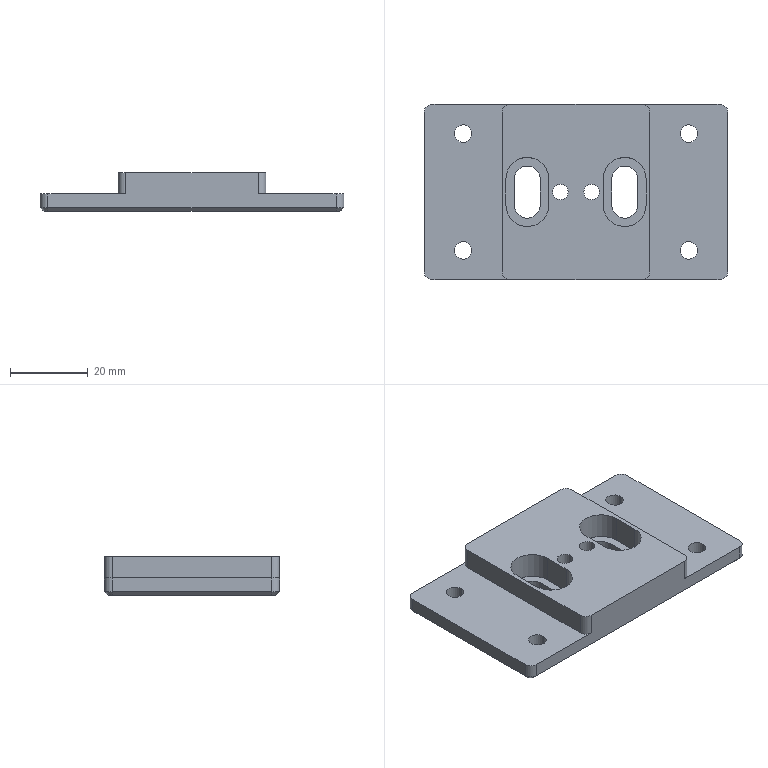NC program | NX | posted with a generic post | part box 78 x 45 x 10 mm
Lines 3249 to 4289 of 4289:
(ZLEVEL_PROFILE_COPY_COPY_1_COPY_1_COPY , TOOL : D4)
N6466 T04 M6
N6468 G54
N6470 G17 G0 G90 X-11.945 Y-4.566 S9500 M3
N6472 G43 Z30. H4
N6474 Z-5.3
N6476 G94 G1 X-11.757 Y-4.479 Z-5.311 F1400.
N6478 X-11.443 Y-4.173 Z-5.334
N6480 X-11.285 Y-3.891 Z-5.351
N6482 X-11.2 Y-3.562 Z-5.369
N6484 Y3.562 Z-5.742
N6486 X-11.285 Y3.891 Z-5.76
N6488 X-11.369 Y4.042 Z-5.769
N6490 X-11.449 Y4.182 Z-5.777
N6492 X-11.764 Y4.484 Z-5.8
N6494 X-12.16 Y4.665 Z-5.823
N6496 X-12.594 Y4.707 Z-5.846
N6498 X-13.017 Y4.604 Z-5.869
N6500 X-13.16 Y4.52 Z-5.877
N6502 X-13.299 Y4.438 Z-5.886
N6504 X-13.553 Y4.179 Z-5.905
N6506 X-13.636 Y4.032 Z-5.914
N6508 X-13.715 Y3.891 Z-5.922
N6510 X-13.8 Y3.562 Z-5.94
N6512 Y-3.562 Z-6.313
N6514 X-13.715 Y-3.891 Z-6.331
N6516 X-13.631 Y-4.041 Z-6.34
N6518 X-13.551 Y-4.182 Z-6.349
N6520 X-13.298 Y-4.439 Z-6.367
N6522 X-13.156 Y-4.522 Z-6.376
N6524 X-13.017 Y-4.604 Z-6.384
N6526 X-12.591 Y-4.707 Z-6.407
N6528 X-12.155 Y-4.664 Z-6.43
N6530 X-11.757 Y-4.479 Z-6.453
N6532 X-11.443 Y-4.173 Z-6.476
N6534 X-11.285 Y-3.891 Z-6.493
N6536 X-11.2 Y-3.562 Z-6.511
N6538 Y3.562 Z-6.884
N6540 X-11.285 Y3.891 Z-6.902
N6542 X-11.369 Y4.042 Z-6.911
N6544 X-11.449 Y4.182 Z-6.92
N6546 X-11.764 Y4.484 Z-6.943
N6548 X-12.16 Y4.665 Z-6.965
N6550 X-12.594 Y4.707 Z-6.988
N6552 X-13.017 Y4.604 Z-7.011
N6554 X-13.16 Y4.52 Z-7.02
N6556 X-13.299 Y4.438 Z-7.028
N6558 X-13.553 Y4.179 Z-7.047
N6560 X-13.636 Y4.032 Z-7.056
N6562 X-13.715 Y3.891 Z-7.065
N6564 X-13.8 Y3.562 Z-7.082
N6566 Y3.4 Z-7.091
N6568 Y-3.4
N6570 G3 X-12.5 Y-4.7 R1.3
N6572 X-11.2 Y-3.4 R1.3
N6574 G1 Y3.4
N6576 G3 X-12.5 Y4.7 R1.3
N6578 X-13.8 Y3.4 R1.3
N6580 G1 Y-3.215 Z-7.209
N6582 X-13.799 Y-3.356 Z-7.211
N6584 X-13.788 Y-3.495 Z-7.214
N6586 X-13.772 Y-3.635 Z-7.216
N6588 X-13.737 Y-3.785 Z-7.219
N6590 X-13.692 Y-3.902 Z-7.221
N6592 X-13.612 Y-4.058 Z-7.224
N6594 X-13.557 Y-4.147 Z-7.226
N6596 X-13.465 Y-4.262 Z-7.229
N6598 X-13.37 Y-4.355 Z-7.231
N6600 X-13.229 Y-4.467 Z-7.235
N6602 X-13.146 Y-4.523 Z-7.236
N6604 X-13.018 Y-4.585 Z-7.239
N6606 X-12.889 Y-4.632 Z-7.241
N6608 X-12.721 Y-4.673 Z-7.244
N6610 X-12.615 Y-4.689 Z-7.246
N6612 X-12.464 Y-4.692 Z-7.249
N6614 X-12.336 Y-4.682 Z-7.251
N6616 X-12.171 Y-4.651 Z-7.254
N6618 X-12.064 Y-4.617 Z-7.256
N6620 X-11.911 Y-4.55 Z-7.259
N6622 X-11.813 Y-4.495 Z-7.261
N6624 X-11.682 Y-4.404 Z-7.264
N6626 X-11.593 Y-4.322 Z-7.266
N6628 X-11.477 Y-4.189 Z-7.27
N6630 X-11.416 Y-4.106 Z-7.271
N6632 X-11.345 Y-3.984 Z-7.274
N6634 X-11.291 Y-3.856 Z-7.276
N6636 X-11.238 Y-3.679 Z-7.28
N6638 X-11.214 Y-3.587 Z-7.282
N6640 X-11.201 Y-3.447 Z-7.284
N6642 X-11.2 Y-3.306 Z-7.287
N6644 Y2.042 Z-7.382
N6646 Y3.4
N6648 G3 X-12.5 Y4.7 R1.3
N6650 X-13.8 Y3.4 R1.3
N6652 G1 Y-3.215 Z-7.5
N6654 X-13.799 Y-3.356 Z-7.502
N6656 X-13.788 Y-3.495 Z-7.505
N6658 X-13.772 Y-3.635 Z-7.507
N6660 X-13.737 Y-3.785 Z-7.51
N6662 X-13.692 Y-3.902 Z-7.512
N6664 X-13.612 Y-4.058 Z-7.515
N6666 X-13.557 Y-4.147 Z-7.517
N6668 X-13.465 Y-4.262 Z-7.52
N6670 X-13.37 Y-4.355 Z-7.522
N6672 X-13.229 Y-4.467 Z-7.525
N6674 X-13.146 Y-4.523 Z-7.527
N6676 X-13.018 Y-4.585 Z-7.53
N6678 X-12.889 Y-4.632 Z-7.532
N6680 X-12.721 Y-4.673 Z-7.535
N6682 X-12.615 Y-4.689 Z-7.537
N6684 X-12.464 Y-4.692 Z-7.54
N6686 X-12.336 Y-4.682 Z-7.542
N6688 X-12.171 Y-4.651 Z-7.545
N6690 X-12.064 Y-4.617 Z-7.547
N6692 X-11.911 Y-4.55 Z-7.55
N6694 X-11.813 Y-4.495 Z-7.552
N6696 X-11.682 Y-4.404 Z-7.555
N6698 X-11.593 Y-4.322 Z-7.557
N6700 X-11.477 Y-4.189 Z-7.561
N6702 X-11.416 Y-4.106 Z-7.562
N6704 X-11.345 Y-3.984 Z-7.565
N6706 X-11.291 Y-3.856 Z-7.567
N6708 X-11.238 Y-3.679 Z-7.571
N6710 X-11.214 Y-3.587 Z-7.572
N6712 X-11.201 Y-3.447 Z-7.575
N6714 X-11.2 Y-3.306 Z-7.577
N6716 Y2.042 Z-7.673
N6718 Y3.4
N6720 G3 X-12.5 Y4.7 R1.3
N6722 X-13.8 Y3.4 R1.3
N6724 G1 Y-3.215 Z-7.791
N6726 X-13.799 Y-3.356 Z-7.793
N6728 X-13.788 Y-3.495 Z-7.796
N6730 X-13.772 Y-3.635 Z-7.798
N6732 X-13.736 Y-3.785 Z-7.801
N6734 X-13.692 Y-3.902 Z-7.803
N6736 X-13.612 Y-4.058 Z-7.806
N6738 X-13.557 Y-4.147 Z-7.808
N6740 X-13.465 Y-4.262 Z-7.811
N6742 X-13.37 Y-4.355 Z-7.813
N6744 X-13.229 Y-4.467 Z-7.816
N6746 X-13.146 Y-4.523 Z-7.818
N6748 X-13.018 Y-4.585 Z-7.821
N6750 X-12.889 Y-4.632 Z-7.823
N6752 X-12.721 Y-4.673 Z-7.826
N6754 X-12.615 Y-4.689 Z-7.828
N6756 X-12.464 Y-4.692 Z-7.831
N6758 X-12.336 Y-4.682 Z-7.833
N6760 X-12.171 Y-4.651 Z-7.836
N6762 X-12.064 Y-4.617 Z-7.838
N6764 X-11.911 Y-4.55 Z-7.841
N6766 X-11.813 Y-4.495 Z-7.843
N6768 X-11.682 Y-4.404 Z-7.846
N6770 X-11.593 Y-4.322 Z-7.848
N6772 X-11.477 Y-4.189 Z-7.851
N6774 X-11.416 Y-4.106 Z-7.853
N6776 X-11.346 Y-3.984 Z-7.856
N6778 X-11.291 Y-3.856 Z-7.858
N6780 X-11.238 Y-3.679 Z-7.862
N6782 X-11.214 Y-3.587 Z-7.863
N6784 X-11.201 Y-3.447 Z-7.866
N6786 X-11.2 Y-3.306 Z-7.868
N6788 Y2.042 Z-7.964
N6790 Y3.4
N6792 G3 X-12.5 Y4.7 R1.3
N6794 X-13.8 Y3.4 R1.3
N6796 G1 Y-3.215 Z-8.082
N6798 X-13.799 Y-3.356 Z-8.084
N6800 X-13.788 Y-3.495 Z-8.087
N6802 X-13.772 Y-3.635 Z-8.089
N6804 X-13.736 Y-3.785 Z-8.092
N6806 X-13.692 Y-3.902 Z-8.094
N6808 X-13.612 Y-4.058 Z-8.097
N6810 X-13.557 Y-4.147 Z-8.099
N6812 X-13.465 Y-4.262 Z-8.102
N6814 X-13.37 Y-4.355 Z-8.104
N6816 X-13.229 Y-4.467 Z-8.107
N6818 X-13.146 Y-4.523 Z-8.109
N6820 X-13.018 Y-4.585 Z-8.112
N6822 X-12.889 Y-4.632 Z-8.114
N6824 X-12.721 Y-4.673 Z-8.117
N6826 X-12.615 Y-4.689 Z-8.119
N6828 X-12.464 Y-4.692 Z-8.122
N6830 X-12.336 Y-4.682 Z-8.124
N6832 X-12.171 Y-4.651 Z-8.127
N6834 X-12.064 Y-4.617 Z-8.129
N6836 X-11.911 Y-4.55 Z-8.132
N6838 X-11.813 Y-4.495 Z-8.134
N6840 X-11.682 Y-4.404 Z-8.137
N6842 X-11.593 Y-4.322 Z-8.139
N6844 X-11.477 Y-4.189 Z-8.142
N6846 X-11.416 Y-4.106 Z-8.144
N6848 X-11.346 Y-3.984 Z-8.147
N6850 X-11.291 Y-3.856 Z-8.149
N6852 X-11.238 Y-3.679 Z-8.153
N6854 X-11.214 Y-3.587 Z-8.154
N6856 X-11.201 Y-3.447 Z-8.157
N6858 X-11.2 Y-3.306 Z-8.159
N6860 Y2.042 Z-8.255
N6862 Y3.4
N6864 G3 X-12.5 Y4.7 R1.3
N6866 X-13.8 Y3.4 R1.3
N6868 G1 Y-3.215 Z-8.372
N6870 X-13.799 Y-3.356 Z-8.375
N6872 X-13.788 Y-3.495 Z-8.377
N6874 X-13.772 Y-3.635 Z-8.38
N6876 X-13.736 Y-3.785 Z-8.383
N6878 X-13.692 Y-3.902 Z-8.385
N6880 X-13.612 Y-4.058 Z-8.388
N6882 X-13.557 Y-4.147 Z-8.39
N6884 X-13.465 Y-4.262 Z-8.393
N6886 X-13.37 Y-4.355 Z-8.395
N6888 X-13.229 Y-4.467 Z-8.398
N6890 X-13.146 Y-4.523 Z-8.4
N6892 X-13.018 Y-4.585 Z-8.403
N6894 X-12.889 Y-4.632 Z-8.405
N6896 X-12.721 Y-4.673 Z-8.408
N6898 X-12.615 Y-4.689 Z-8.41
N6900 X-12.464 Y-4.692 Z-8.413
N6902 X-12.336 Y-4.682 Z-8.415
N6904 X-12.171 Y-4.651 Z-8.418
N6906 X-12.064 Y-4.617 Z-8.42
N6908 X-11.911 Y-4.55 Z-8.423
N6910 X-11.813 Y-4.495 Z-8.425
N6912 X-11.682 Y-4.404 Z-8.428
N6914 X-11.593 Y-4.322 Z-8.43
N6916 X-11.477 Y-4.189 Z-8.433
N6918 X-11.416 Y-4.106 Z-8.435
N6920 X-11.346 Y-3.984 Z-8.438
N6922 X-11.291 Y-3.856 Z-8.44
N6924 X-11.238 Y-3.679 Z-8.443
N6926 X-11.214 Y-3.587 Z-8.445
N6928 X-11.201 Y-3.447 Z-8.448
N6930 X-11.2 Y-3.306 Z-8.45
N6932 Y2.042 Z-8.545
N6934 Y3.4
N6936 G3 X-12.5 Y4.7 R1.3
N6938 X-13.8 Y3.4 R1.3
N6940 G1 Y-3.215 Z-8.663
N6942 X-13.799 Y-3.356 Z-8.666
N6944 X-13.788 Y-3.495 Z-8.668
N6946 X-13.772 Y-3.635 Z-8.671
N6948 X-13.736 Y-3.785 Z-8.674
N6950 X-13.692 Y-3.902 Z-8.676
N6952 X-13.612 Y-4.058 Z-8.679
N6954 X-13.557 Y-4.147 Z-8.681
N6956 X-13.465 Y-4.262 Z-8.684
N6958 X-13.37 Y-4.355 Z-8.686
N6960 X-13.229 Y-4.467 Z-8.689
N6962 X-13.146 Y-4.523 Z-8.691
N6964 X-13.018 Y-4.585 Z-8.693
N6966 X-12.889 Y-4.632 Z-8.696
N6968 X-12.721 Y-4.673 Z-8.699
N6970 X-12.615 Y-4.689 Z-8.701
N6972 X-12.464 Y-4.692 Z-8.704
N6974 X-12.336 Y-4.682 Z-8.706
N6976 X-12.171 Y-4.651 Z-8.709
N6978 X-12.064 Y-4.617 Z-8.711
N6980 X-11.911 Y-4.55 Z-8.714
N6982 X-11.813 Y-4.495 Z-8.716
N6984 X-11.682 Y-4.404 Z-8.719
N6986 X-11.593 Y-4.322 Z-8.721
N6988 X-11.477 Y-4.189 Z-8.724
N6990 X-11.416 Y-4.106 Z-8.726
N6992 X-11.346 Y-3.984 Z-8.729
N6994 X-11.291 Y-3.856 Z-8.731
N6996 X-11.238 Y-3.679 Z-8.734
N6998 X-11.214 Y-3.587 Z-8.736
N7000 X-11.201 Y-3.447 Z-8.739
N7002 X-11.2 Y-3.306 Z-8.741
N7004 Y2.042 Z-8.836
N7006 Y3.4
N7008 G3 X-12.5 Y4.7 R1.3
N7010 X-13.8 Y3.4 R1.3
N7012 G1 Y-3.215 Z-8.954
N7014 X-13.799 Y-3.356 Z-8.957
N7016 X-13.788 Y-3.495 Z-8.959
N7018 X-13.772 Y-3.635 Z-8.962
N7020 X-13.736 Y-3.785 Z-8.965
N7022 X-13.692 Y-3.902 Z-8.967
N7024 X-13.612 Y-4.058 Z-8.97
N7026 X-13.557 Y-4.147 Z-8.972
N7028 X-13.465 Y-4.262 Z-8.974
N7030 X-13.37 Y-4.355 Z-8.977
N7032 X-13.229 Y-4.467 Z-8.98
N7034 X-13.146 Y-4.523 Z-8.982
N7036 X-13.018 Y-4.585 Z-8.984
N7038 X-12.889 Y-4.632 Z-8.987
N7040 X-12.721 Y-4.673 Z-8.99
N7042 X-12.615 Y-4.689 Z-8.992
N7044 X-12.464 Y-4.692 Z-8.995
N7046 X-12.336 Y-4.682 Z-8.997
N7048 X-12.171 Y-4.651 Z-9.
N7050 X-12.064 Y-4.617 Z-9.002
N7052 X-11.911 Y-4.55 Z-9.005
N7054 X-11.813 Y-4.495 Z-9.007
N7056 X-11.682 Y-4.404 Z-9.01
N7058 X-11.593 Y-4.322 Z-9.012
N7060 X-11.477 Y-4.19 Z-9.015
N7062 X-11.416 Y-4.106 Z-9.017
N7064 X-11.346 Y-3.984 Z-9.019
N7066 X-11.291 Y-3.856 Z-9.022
N7068 X-11.238 Y-3.679 Z-9.025
N7070 X-11.214 Y-3.587 Z-9.027
N7072 X-11.201 Y-3.447 Z-9.029
N7074 X-11.2 Y-3.306 Z-9.032
N7076 Y2.042 Z-9.127
N7078 Y3.4
N7080 G3 X-12.5 Y4.7 R1.3
N7082 X-13.8 Y3.4 R1.3
N7084 G1 Y-3.215 Z-9.245
N7086 X-13.799 Y-3.356 Z-9.248
N7088 X-13.788 Y-3.495 Z-9.25
N7090 X-13.772 Y-3.635 Z-9.253
N7092 X-13.736 Y-3.785 Z-9.255
N7094 X-13.692 Y-3.902 Z-9.258
N7096 X-13.612 Y-4.058 Z-9.261
N7098 X-13.557 Y-4.147 Z-9.263
N7100 X-13.465 Y-4.262 Z-9.265
N7102 X-13.37 Y-4.355 Z-9.268
N7104 X-13.229 Y-4.467 Z-9.271
N7106 X-13.146 Y-4.523 Z-9.273
N7108 X-13.018 Y-4.585 Z-9.275
N7110 X-12.889 Y-4.632 Z-9.278
N7112 X-12.721 Y-4.673 Z-9.281
N7114 X-12.615 Y-4.689 Z-9.283
N7116 X-12.464 Y-4.692 Z-9.285
N7118 X-12.336 Y-4.682 Z-9.288
N7120 X-12.171 Y-4.651 Z-9.291
N7122 X-12.064 Y-4.617 Z-9.293
N7124 X-11.911 Y-4.55 Z-9.296
N7126 X-11.813 Y-4.495 Z-9.298
N7128 X-11.682 Y-4.404 Z-9.301
N7130 X-11.593 Y-4.322 Z-9.303
N7132 X-11.477 Y-4.19 Z-9.306
N7134 X-11.416 Y-4.106 Z-9.308
N7136 X-11.346 Y-3.984 Z-9.31
N7138 X-11.291 Y-3.856 Z-9.313
N7140 X-11.238 Y-3.679 Z-9.316
N7142 X-11.214 Y-3.587 Z-9.318
N7144 X-11.201 Y-3.447 Z-9.32
N7146 X-11.2 Y-3.306 Z-9.323
N7148 Y2.042 Z-9.418
N7150 Y3.4
N7152 G3 X-12.5 Y4.7 R1.3
N7154 X-13.8 Y3.4 R1.3
N7156 G1 Y-3.215 Z-9.536
N7158 X-13.799 Y-3.356 Z-9.539
N7160 X-13.788 Y-3.495 Z-9.541
N7162 X-13.772 Y-3.635 Z-9.544
N7164 X-13.736 Y-3.785 Z-9.546
N7166 X-13.692 Y-3.902 Z-9.549
N7168 X-13.612 Y-4.058 Z-9.552
N7170 X-13.557 Y-4.147 Z-9.554
N7172 X-13.465 Y-4.262 Z-9.556
N7174 X-13.37 Y-4.355 Z-9.559
N7176 X-13.229 Y-4.467 Z-9.562
N7178 X-13.146 Y-4.523 Z-9.564
N7180 X-13.018 Y-4.585 Z-9.566
N7182 X-12.889 Y-4.632 Z-9.569
N7184 X-12.721 Y-4.673 Z-9.572
N7186 X-12.615 Y-4.689 Z-9.574
N7188 X-12.464 Y-4.692 Z-9.576
N7190 X-12.336 Y-4.682 Z-9.579
N7192 X-12.171 Y-4.651 Z-9.582
N7194 X-12.064 Y-4.617 Z-9.584
N7196 X-11.911 Y-4.55 Z-9.587
N7198 X-11.813 Y-4.495 Z-9.589
N7200 X-11.682 Y-4.404 Z-9.592
N7202 X-11.593 Y-4.322 Z-9.594
N7204 X-11.477 Y-4.19 Z-9.597
N7206 X-11.416 Y-4.106 Z-9.599
N7208 X-11.346 Y-3.985 Z-9.601
N7210 X-11.291 Y-3.856 Z-9.604
N7212 X-11.238 Y-3.679 Z-9.607
N7214 X-11.214 Y-3.587 Z-9.609
N7216 X-11.201 Y-3.447 Z-9.611
N7218 X-11.2 Y-3.306 Z-9.614
N7220 Y2.042 Z-9.709
N7222 Y3.4
N7224 G3 X-12.5 Y4.7 R1.3
N7226 X-13.8 Y3.4 R1.3
N7228 G1 Y-3.215 Z-9.827
N7230 X-13.799 Y-3.356 Z-9.829
N7232 X-13.788 Y-3.495 Z-9.832
N7234 X-13.772 Y-3.635 Z-9.834
N7236 X-13.736 Y-3.785 Z-9.837
N7238 X-13.692 Y-3.902 Z-9.839
N7240 X-13.612 Y-4.058 Z-9.843
N7242 X-13.557 Y-4.147 Z-9.845
N7244 X-13.465 Y-4.262 Z-9.847
N7246 X-13.37 Y-4.355 Z-9.85
N7248 X-13.229 Y-4.467 Z-9.853
N7250 X-13.146 Y-4.523 Z-9.855
N7252 X-13.018 Y-4.585 Z-9.857
N7254 X-12.889 Y-4.632 Z-9.86
N7256 X-12.721 Y-4.673 Z-9.863
N7258 X-12.615 Y-4.689 Z-9.865
N7260 X-12.464 Y-4.692 Z-9.867
N7262 X-12.336 Y-4.682 Z-9.87
N7264 X-12.171 Y-4.651 Z-9.873
N7266 X-12.064 Y-4.617 Z-9.875
N7268 X-11.911 Y-4.55 Z-9.878
N7270 X-11.813 Y-4.495 Z-9.88
N7272 X-11.682 Y-4.404 Z-9.882
N7274 X-11.593 Y-4.322 Z-9.885
N7276 X-11.478 Y-4.19 Z-9.888
N7278 X-11.416 Y-4.106 Z-9.89
N7280 X-11.346 Y-3.985 Z-9.892
N7282 X-11.291 Y-3.856 Z-9.895
N7284 X-11.238 Y-3.679 Z-9.898
N7286 X-11.214 Y-3.587 Z-9.9
N7288 X-11.201 Y-3.447 Z-9.902
N7290 X-11.2 Y-3.306 Z-9.905
N7292 Y2.042 Z-10.
N7294 Y3.4
N7296 G3 X-12.5 Y4.7 R1.3
N7298 X-13.8 Y3.4 R1.3
N7300 G1 Y-3.4
N7302 G3 X-12.5 Y-4.7 R1.3
N7304 X-11.2 Y-3.4 R1.3
N7306 G1 Y2.042
N7308 G3 X-11.4 Y2.388 R0.4
N7310 G1 X-11.7 Y2.562
N7312 Z-9.6
N7314 G0 Z30.
N7316 X13.055 Y-4.566
N7318 Z-5.3
N7320 G1 X13.243 Y-4.479 Z-5.311
N7322 X13.557 Y-4.173 Z-5.334
N7324 X13.715 Y-3.891 Z-5.351
N7326 X13.8 Y-3.562 Z-5.369
N7328 Y3.562 Z-5.742
N7330 X13.715 Y3.891 Z-5.76
N7332 X13.631 Y4.042 Z-5.769
N7334 X13.551 Y4.182 Z-5.777
N7336 X13.236 Y4.484 Z-5.8
N7338 X12.84 Y4.665 Z-5.823
N7340 X12.406 Y4.707 Z-5.846
N7342 X11.983 Y4.604 Z-5.869
N7344 X11.84 Y4.52 Z-5.877
N7346 X11.701 Y4.438 Z-5.886
N7348 X11.447 Y4.179 Z-5.905
N7350 X11.364 Y4.032 Z-5.914
N7352 X11.285 Y3.891 Z-5.922
N7354 X11.2 Y3.562 Z-5.94
N7356 Y-3.562 Z-6.313
N7358 X11.285 Y-3.891 Z-6.331
N7360 X11.369 Y-4.041 Z-6.34
N7362 X11.449 Y-4.182 Z-6.349
N7364 X11.702 Y-4.439 Z-6.367
N7366 X11.844 Y-4.522 Z-6.376
N7368 X11.983 Y-4.604 Z-6.384
N7370 X12.409 Y-4.707 Z-6.407
N7372 X12.845 Y-4.664 Z-6.43
N7374 X13.243 Y-4.479 Z-6.453
N7376 X13.557 Y-4.173 Z-6.476
N7378 X13.715 Y-3.891 Z-6.493
N7380 X13.8 Y-3.562 Z-6.511
N7382 Y3.562 Z-6.884
N7384 X13.715 Y3.891 Z-6.902
N7386 X13.631 Y4.042 Z-6.911
N7388 X13.551 Y4.182 Z-6.92
N7390 X13.236 Y4.484 Z-6.943
N7392 X12.84 Y4.665 Z-6.965
N7394 X12.406 Y4.707 Z-6.988
N7396 X11.983 Y4.604 Z-7.011
N7398 X11.84 Y4.52 Z-7.02
N7400 X11.701 Y4.438 Z-7.028
N7402 X11.447 Y4.179 Z-7.047
N7404 X11.364 Y4.032 Z-7.056
N7406 X11.285 Y3.891 Z-7.065
N7408 X11.2 Y3.562 Z-7.082
N7410 Y3.4 Z-7.091
N7412 Y-3.4
N7414 G3 X12.5 Y-4.7 R1.3
N7416 X13.8 Y-3.4 R1.3
N7418 G1 Y3.4
N7420 G3 X12.5 Y4.7 R1.3
N7422 X11.2 Y3.4 R1.3
N7424 G1 Y-3.356 Z-7.211
N7426 X11.211 Y-3.495 Z-7.214
N7428 X11.228 Y-3.635 Z-7.216
N7430 X11.264 Y-3.787 Z-7.219
N7432 X11.308 Y-3.902 Z-7.221
N7434 X11.389 Y-4.059 Z-7.224
N7436 X11.443 Y-4.147 Z-7.226
N7438 X11.535 Y-4.262 Z-7.229
N7440 X11.63 Y-4.355 Z-7.231
N7442 X11.771 Y-4.467 Z-7.235
N7444 X11.854 Y-4.523 Z-7.236
N7446 X11.982 Y-4.585 Z-7.239
N7448 X12.111 Y-4.632 Z-7.241
N7450 X12.279 Y-4.673 Z-7.244
N7452 X12.385 Y-4.689 Z-7.246
N7454 X12.536 Y-4.692 Z-7.249
N7456 X12.664 Y-4.682 Z-7.251
N7458 X12.829 Y-4.651 Z-7.254
N7460 X12.936 Y-4.617 Z-7.256
N7462 X13.089 Y-4.55 Z-7.259
N7464 X13.187 Y-4.495 Z-7.261
N7466 X13.318 Y-4.404 Z-7.264
N7468 X13.407 Y-4.322 Z-7.266
N7470 X13.523 Y-4.189 Z-7.27
N7472 X13.584 Y-4.106 Z-7.271
N7474 X13.657 Y-3.979 Z-7.274
N7476 X13.709 Y-3.856 Z-7.276
N7478 X13.758 Y-3.696 Z-7.279
N7480 X13.782 Y-3.586 Z-7.282
N7482 X13.793 Y-3.446 Z-7.284
N7484 X13.8 Y-3.306 Z-7.287
N7486 Y2.042 Z-7.382
N7488 Y3.4
N7490 G3 X12.5 Y4.7 R1.3
N7492 X11.2 Y3.4 R1.3
N7494 G1 Y-3.356 Z-7.502
N7496 X11.211 Y-3.495 Z-7.505
N7498 X11.228 Y-3.635 Z-7.507
N7500 X11.264 Y-3.787 Z-7.51
N7502 X11.308 Y-3.902 Z-7.512
N7504 X11.389 Y-4.059 Z-7.515
N7506 X11.443 Y-4.147 Z-7.517
N7508 X11.535 Y-4.262 Z-7.52
N7510 X11.63 Y-4.355 Z-7.522
N7512 X11.771 Y-4.467 Z-7.525
N7514 X11.854 Y-4.523 Z-7.527
N7516 X11.982 Y-4.585 Z-7.53
N7518 X12.111 Y-4.632 Z-7.532
N7520 X12.279 Y-4.673 Z-7.535
N7522 X12.385 Y-4.689 Z-7.537
N7524 X12.536 Y-4.692 Z-7.54
N7526 X12.664 Y-4.682 Z-7.542
N7528 X12.829 Y-4.651 Z-7.545
N7530 X12.936 Y-4.617 Z-7.547
N7532 X13.089 Y-4.55 Z-7.55
N7534 X13.187 Y-4.495 Z-7.552
N7536 X13.318 Y-4.404 Z-7.555
N7538 X13.407 Y-4.322 Z-7.557
N7540 X13.523 Y-4.189 Z-7.561
N7542 X13.584 Y-4.106 Z-7.562
N7544 X13.657 Y-3.979 Z-7.565
N7546 X13.709 Y-3.856 Z-7.567
N7548 X13.758 Y-3.696 Z-7.57
N7550 X13.782 Y-3.586 Z-7.572
N7552 X13.793 Y-3.446 Z-7.575
N7554 X13.8 Y-3.306 Z-7.577
N7556 Y2.042 Z-7.673
N7558 Y3.4
N7560 G3 X12.5 Y4.7 R1.3
N7562 X11.2 Y3.4 R1.3
N7564 G1 Y-3.356 Z-7.793
N7566 X11.211 Y-3.495 Z-7.796
N7568 X11.228 Y-3.635 Z-7.798
N7570 X11.264 Y-3.787 Z-7.801
N7572 X11.308 Y-3.902 Z-7.803
N7574 X11.389 Y-4.059 Z-7.806
N7576 X11.443 Y-4.147 Z-7.808
N7578 X11.535 Y-4.262 Z-7.811
N7580 X11.63 Y-4.355 Z-7.813
N7582 X11.771 Y-4.467 Z-7.816
N7584 X11.854 Y-4.523 Z-7.818
N7586 X11.982 Y-4.585 Z-7.821
N7588 X12.111 Y-4.632 Z-7.823
N7590 X12.279 Y-4.673 Z-7.826
N7592 X12.385 Y-4.689 Z-7.828
N7594 X12.536 Y-4.692 Z-7.831
N7596 X12.664 Y-4.682 Z-7.833
N7598 X12.829 Y-4.651 Z-7.836
N7600 X12.936 Y-4.617 Z-7.838
N7602 X13.089 Y-4.55 Z-7.841
N7604 X13.187 Y-4.495 Z-7.843
N7606 X13.318 Y-4.404 Z-7.846
N7608 X13.407 Y-4.322 Z-7.848
N7610 X13.523 Y-4.189 Z-7.851
N7612 X13.584 Y-4.106 Z-7.853
N7614 X13.657 Y-3.979 Z-7.856
N7616 X13.709 Y-3.856 Z-7.858
N7618 X13.758 Y-3.696 Z-7.861
N7620 X13.782 Y-3.586 Z-7.863
N7622 X13.793 Y-3.446 Z-7.866
N7624 X13.8 Y-3.306 Z-7.868
N7626 Y2.042 Z-7.964
N7628 Y3.4
N7630 G3 X12.5 Y4.7 R1.3
N7632 X11.2 Y3.4 R1.3
N7634 G1 Y-3.356 Z-8.084
N7636 X11.211 Y-3.495 Z-8.087
N7638 X11.228 Y-3.635 Z-8.089
N7640 X11.264 Y-3.787 Z-8.092
N7642 X11.308 Y-3.902 Z-8.094
N7644 X11.389 Y-4.058 Z-8.097
N7646 X11.443 Y-4.147 Z-8.099
N7648 X11.535 Y-4.262 Z-8.102
N7650 X11.63 Y-4.355 Z-8.104
N7652 X11.771 Y-4.467 Z-8.107
N7654 X11.854 Y-4.523 Z-8.109
N7656 X11.982 Y-4.585 Z-8.112
N7658 X12.111 Y-4.632 Z-8.114
N7660 X12.279 Y-4.673 Z-8.117
N7662 X12.385 Y-4.689 Z-8.119
N7664 X12.536 Y-4.692 Z-8.122
N7666 X12.664 Y-4.682 Z-8.124
N7668 X12.829 Y-4.651 Z-8.127
N7670 X12.936 Y-4.617 Z-8.129
N7672 X13.089 Y-4.55 Z-8.132
N7674 X13.187 Y-4.495 Z-8.134
N7676 X13.318 Y-4.404 Z-8.137
N7678 X13.407 Y-4.322 Z-8.139
N7680 X13.523 Y-4.189 Z-8.142
N7682 X13.584 Y-4.106 Z-8.144
N7684 X13.657 Y-3.979 Z-8.147
N7686 X13.709 Y-3.856 Z-8.149
N7688 X13.758 Y-3.696 Z-8.152
N7690 X13.782 Y-3.586 Z-8.154
N7692 X13.793 Y-3.446 Z-8.157
N7694 X13.8 Y-3.306 Z-8.159
N7696 Y2.042 Z-8.255
N7698 Y3.4
N7700 G3 X12.5 Y4.7 R1.3
N7702 X11.2 Y3.4 R1.3
N7704 G1 Y-3.356 Z-8.375
N7706 X11.211 Y-3.495 Z-8.377
N7708 X11.228 Y-3.635 Z-8.38
N7710 X11.264 Y-3.787 Z-8.383
N7712 X11.308 Y-3.902 Z-8.385
N7714 X11.389 Y-4.058 Z-8.388
N7716 X11.443 Y-4.147 Z-8.39
N7718 X11.535 Y-4.262 Z-8.393
N7720 X11.63 Y-4.355 Z-8.395
N7722 X11.771 Y-4.467 Z-8.398
N7724 X11.854 Y-4.523 Z-8.4
N7726 X11.982 Y-4.585 Z-8.403
N7728 X12.111 Y-4.632 Z-8.405
N7730 X12.279 Y-4.673 Z-8.408
N7732 X12.385 Y-4.689 Z-8.41
N7734 X12.536 Y-4.692 Z-8.413
N7736 X12.664 Y-4.682 Z-8.415
N7738 X12.829 Y-4.651 Z-8.418
N7740 X12.936 Y-4.617 Z-8.42
N7742 X13.089 Y-4.55 Z-8.423
N7744 X13.187 Y-4.495 Z-8.425
N7746 X13.318 Y-4.404 Z-8.428
N7748 X13.407 Y-4.322 Z-8.43
N7750 X13.523 Y-4.189 Z-8.433
N7752 X13.584 Y-4.106 Z-8.435
N7754 X13.657 Y-3.979 Z-8.438
N7756 X13.709 Y-3.856 Z-8.44
N7758 X13.758 Y-3.696 Z-8.443
N7760 X13.782 Y-3.586 Z-8.445
N7762 X13.793 Y-3.446 Z-8.448
N7764 X13.8 Y-3.306 Z-8.45
N7766 Y2.042 Z-8.545
N7768 Y3.4
N7770 G3 X12.5 Y4.7 R1.3
N7772 X11.2 Y3.4 R1.3
N7774 G1 Y-3.356 Z-8.666
N7776 X11.211 Y-3.495 Z-8.668
N7778 X11.228 Y-3.635 Z-8.671
N7780 X11.264 Y-3.787 Z-8.674
N7782 X11.308 Y-3.902 Z-8.676
N7784 X11.389 Y-4.058 Z-8.679
N7786 X11.443 Y-4.147 Z-8.681
N7788 X11.535 Y-4.262 Z-8.684
N7790 X11.63 Y-4.355 Z-8.686
N7792 X11.771 Y-4.467 Z-8.689
N7794 X11.854 Y-4.523 Z-8.691
N7796 X11.982 Y-4.585 Z-8.693
N7798 X12.111 Y-4.632 Z-8.696
N7800 X12.279 Y-4.673 Z-8.699
N7802 X12.385 Y-4.689 Z-8.701
N7804 X12.536 Y-4.692 Z-8.704
N7806 X12.664 Y-4.682 Z-8.706
N7808 X12.829 Y-4.651 Z-8.709
N7810 X12.936 Y-4.617 Z-8.711
N7812 X13.089 Y-4.55 Z-8.714
N7814 X13.187 Y-4.495 Z-8.716
N7816 X13.318 Y-4.404 Z-8.719
N7818 X13.407 Y-4.322 Z-8.721
N7820 X13.523 Y-4.189 Z-8.724
N7822 X13.584 Y-4.106 Z-8.726
N7824 X13.657 Y-3.979 Z-8.729
N7826 X13.709 Y-3.856 Z-8.731
N7828 X13.758 Y-3.696 Z-8.734
N7830 X13.782 Y-3.586 Z-8.736
N7832 X13.793 Y-3.446 Z-8.739
N7834 X13.8 Y-3.306 Z-8.741
N7836 Y2.042 Z-8.836
N7838 Y3.4
N7840 G3 X12.5 Y4.7 R1.3
N7842 X11.2 Y3.4 R1.3
N7844 G1 Y-3.356 Z-8.957
N7846 X11.211 Y-3.495 Z-8.959
N7848 X11.228 Y-3.635 Z-8.962
N7850 X11.264 Y-3.787 Z-8.965
N7852 X11.308 Y-3.902 Z-8.967
N7854 X11.389 Y-4.058 Z-8.97
N7856 X11.443 Y-4.147 Z-8.972
N7858 X11.535 Y-4.262 Z-8.974
N7860 X11.63 Y-4.355 Z-8.977
N7862 X11.771 Y-4.467 Z-8.98
N7864 X11.854 Y-4.523 Z-8.982
N7866 X11.982 Y-4.585 Z-8.984
N7868 X12.111 Y-4.632 Z-8.987
N7870 X12.279 Y-4.673 Z-8.99
N7872 X12.385 Y-4.689 Z-8.992
N7874 X12.536 Y-4.692 Z-8.995
N7876 X12.664 Y-4.682 Z-8.997
N7878 X12.829 Y-4.651 Z-9.
N7880 X12.936 Y-4.617 Z-9.002
N7882 X13.089 Y-4.55 Z-9.005
N7884 X13.187 Y-4.495 Z-9.007
N7886 X13.318 Y-4.404 Z-9.01
N7888 X13.407 Y-4.322 Z-9.012
N7890 X13.523 Y-4.19 Z-9.015
N7892 X13.584 Y-4.106 Z-9.017
N7894 X13.658 Y-3.979 Z-9.02
N7896 X13.709 Y-3.856 Z-9.022
N7898 X13.759 Y-3.692 Z-9.025
N7900 X13.782 Y-3.586 Z-9.027
N7902 X13.793 Y-3.446 Z-9.029
N7904 X13.8 Y-3.306 Z-9.032
N7906 Y2.042 Z-9.127
N7908 Y3.4
N7910 G3 X12.5 Y4.7 R1.3
N7912 X11.2 Y3.4 R1.3
N7914 G1 Y-3.356 Z-9.248
N7916 X11.211 Y-3.495 Z-9.25
N7918 X11.228 Y-3.635 Z-9.253
N7920 X11.264 Y-3.787 Z-9.255
N7922 X11.308 Y-3.902 Z-9.258
N7924 X11.389 Y-4.058 Z-9.261
N7926 X11.443 Y-4.147 Z-9.263
N7928 X11.535 Y-4.262 Z-9.265
N7930 X11.63 Y-4.355 Z-9.268
N7932 X11.771 Y-4.467 Z-9.271
N7934 X11.854 Y-4.523 Z-9.273
N7936 X11.982 Y-4.585 Z-9.275
N7938 X12.111 Y-4.632 Z-9.278
N7940 X12.279 Y-4.673 Z-9.281
N7942 X12.385 Y-4.689 Z-9.283
N7944 X12.536 Y-4.692 Z-9.285
N7946 X12.664 Y-4.682 Z-9.288
N7948 X12.829 Y-4.651 Z-9.291
N7950 X12.936 Y-4.617 Z-9.293
N7952 X13.089 Y-4.55 Z-9.296
N7954 X13.187 Y-4.495 Z-9.298
N7956 X13.318 Y-4.404 Z-9.301
N7958 X13.407 Y-4.322 Z-9.303
N7960 X13.523 Y-4.19 Z-9.306
N7962 X13.584 Y-4.106 Z-9.308
N7964 X13.658 Y-3.979 Z-9.31
N7966 X13.709 Y-3.856 Z-9.313
N7968 X13.759 Y-3.692 Z-9.316
N7970 X13.782 Y-3.586 Z-9.318
N7972 X13.793 Y-3.446 Z-9.32
N7974 X13.8 Y-3.306 Z-9.323
N7976 Y2.042 Z-9.418
N7978 Y3.4
N7980 G3 X12.5 Y4.7 R1.3
N7982 X11.2 Y3.4 R1.3
N7984 G1 Y-3.356 Z-9.539
N7986 X11.211 Y-3.495 Z-9.541
N7988 X11.228 Y-3.635 Z-9.544
N7990 X11.264 Y-3.787 Z-9.546
N7992 X11.308 Y-3.902 Z-9.549
N7994 X11.389 Y-4.058 Z-9.552
N7996 X11.443 Y-4.147 Z-9.554
N7998 X11.535 Y-4.262 Z-9.556
N8000 X11.63 Y-4.355 Z-9.559
N8002 X11.771 Y-4.467 Z-9.562
N8004 X11.854 Y-4.523 Z-9.564
N8006 X11.982 Y-4.585 Z-9.566
N8008 X12.111 Y-4.632 Z-9.569
N8010 X12.279 Y-4.673 Z-9.572
N8012 X12.385 Y-4.689 Z-9.574
N8014 X12.536 Y-4.692 Z-9.576
N8016 X12.664 Y-4.682 Z-9.579
N8018 X12.829 Y-4.651 Z-9.582
N8020 X12.936 Y-4.617 Z-9.584
N8022 X13.089 Y-4.55 Z-9.587
N8024 X13.187 Y-4.495 Z-9.589
N8026 X13.318 Y-4.404 Z-9.592
N8028 X13.407 Y-4.322 Z-9.594
N8030 X13.523 Y-4.19 Z-9.597
N8032 X13.584 Y-4.106 Z-9.599
N8034 X13.658 Y-3.979 Z-9.601
N8036 X13.709 Y-3.856 Z-9.604
N8038 X13.759 Y-3.692 Z-9.607
N8040 X13.782 Y-3.586 Z-9.609
N8042 X13.793 Y-3.446 Z-9.611
N8044 X13.8 Y-3.306 Z-9.614
N8046 Y2.042 Z-9.709
N8048 Y3.4
N8050 G3 X12.5 Y4.7 R1.3
N8052 X11.2 Y3.4 R1.3
N8054 G1 Y-3.356 Z-9.829
N8056 X11.211 Y-3.495 Z-9.832
N8058 X11.228 Y-3.635 Z-9.834
N8060 X11.264 Y-3.787 Z-9.837
N8062 X11.308 Y-3.902 Z-9.839
N8064 X11.389 Y-4.058 Z-9.843
N8066 X11.443 Y-4.147 Z-9.845
N8068 X11.535 Y-4.262 Z-9.847
N8070 X11.63 Y-4.355 Z-9.85
N8072 X11.771 Y-4.467 Z-9.853
N8074 X11.854 Y-4.523 Z-9.855
N8076 X11.982 Y-4.585 Z-9.857
N8078 X12.111 Y-4.632 Z-9.86
N8080 X12.279 Y-4.673 Z-9.863
N8082 X12.385 Y-4.689 Z-9.865
N8084 X12.536 Y-4.692 Z-9.867
N8086 X12.664 Y-4.682 Z-9.87
N8088 X12.829 Y-4.651 Z-9.873
N8090 X12.936 Y-4.617 Z-9.875
N8092 X13.089 Y-4.55 Z-9.878
N8094 X13.187 Y-4.495 Z-9.88
N8096 X13.318 Y-4.404 Z-9.882
N8098 X13.407 Y-4.322 Z-9.885
N8100 X13.522 Y-4.19 Z-9.888
N8102 X13.584 Y-4.106 Z-9.89
N8104 X13.658 Y-3.979 Z-9.892
N8106 X13.709 Y-3.856 Z-9.895
N8108 X13.759 Y-3.692 Z-9.898
N8110 X13.782 Y-3.586 Z-9.9
N8112 X13.793 Y-3.446 Z-9.902
N8114 X13.8 Y-3.306 Z-9.905
N8116 Y2.042 Z-10.
N8118 Y3.4
N8120 G3 X12.5 Y4.7 R1.3
N8122 X11.2 Y3.4 R1.3
N8124 G1 Y-3.4
N8126 G3 X12.5 Y-4.7 R1.3
N8128 X13.8 Y-3.4 R1.3
N8130 G1 Y2.042
N8132 G3 X13.6 Y2.388 R0.4
N8134 G1 X13.3 Y2.562
N8136 Z-9.6
N8138 G0 Z30.
N8140 M5
(DRILLING_COPY_1 , TOOL : D6A45)
N8142 T07 M6
N8144 G54
N8146 G17 G0 G90 X-29. Y-15. S5000 M3
N8148 G43 Z30. H7
N8150 G94 G81 G98 Z-6.5 F250. R-2.5
N8152 Y15.
N8154 X-4. Y0. Z-1. R3.
N8156 X4.
N8158 X29. Y-15. Z-6.5 R-2.5
N8160 Y15.
N8162 G80
N8164 G0 X29. Y15. Z30.
N8166 M5
(DRILLING_COPY_COPY_1 , TOOL : 4.5ZT)
N8168 T16 M6
N8170 G54
N8172 G17 G0 G90 X-29. Y-15. S2000 M3
N8174 G43 Z30. H16
N8176 G94 G83 G98 Z-12.852 F150. Q2. R-2.5
N8178 Y15.
N8180 X29.
N8182 Y-15.
N8184 G80
N8186 G0 X29. Y-15. Z30.
N8188 M5
(DRILLING_COPY_COPY_1_1 , TOOL : 3.8ZT)
N8190 T13 M6
N8192 G54
N8194 G17 G0 G90 X-4. Y0. S2000 M3
N8196 G43 Z30. H13
N8198 G94 G83 G98 Z-12.642 F150. Q2. R3.
N8200 X4.
N8202 G80
N8204 G0 X4. Y0. Z30.
N8206 M5
(DRILLING_COPY_COPY_1_COPY , TOOL : 4.0JD)
N8208 T12 M6
N8210 G54
N8212 G17 G0 G90 X-4. Y0. S1000 M3
N8214 G43 Z30. H12
N8216 G94 G85 G98 Z-10.5 F50. R3.
N8218 X4.
N8220 G80
N8222 G0 X4. Y0. Z30.
N8224 M5
(ZLEVEL_PROFILE_1_COPY_1_COPY , TOOL : D6A45)
N8226 T07 M6
N8228 G54
N8230 G17 G0 G90 X-4. Y1.041 S9500 M3
N8232 G43 Z30. H7
N8234 Z1.
N8236 G94 G1 Z-1. F1000.
N8238 G3 X-5.041 Y0. R1.041
N8240 X-4. Y1.041 R-1.041
N8242 X-4.52 Y0.741 R0.6
N8244 G1 Z0.
N8246 G0 Z30.
N8248 X-9.366 Y-4.559
N8250 Z0.
N8252 G1 Z-1.
N8254 X-8.259 Y-3.92
N8256 G3 X-7.959 Y-3.4 R0.6
N8258 G1 Y3.4
N8260 G3 X-12.5 Y7.941 R4.541
N8262 X-17.041 Y3.4 R4.541
N8264 G1 Y-3.4
N8266 G3 X-12.5 Y-7.941 R4.541
N8268 X-7.959 Y-3.4 R4.541
N8270 X-8.259 Y-2.88 R0.6
N8272 G1 X-9.159 Y-2.361
N8274 Z0.
N8276 G0 Z30.
N8278 X9.366 Y4.559
N8280 Z0.
N8282 G1 Z-1.
N8284 X8.259 Y3.92
N8286 G3 X7.959 Y3.4 R0.6
N8288 G1 Y-3.4
N8290 G3 X12.5 Y-7.941 R4.541
N8292 X17.041 Y-3.4 R4.541
N8294 G1 Y3.4
N8296 G3 X12.5 Y7.941 R4.541
N8298 X7.959 Y3.4 R4.541
N8300 X8.259 Y2.88 R0.6
N8302 G1 X9.159 Y2.361
N8304 Z0.
N8306 G0 Z30.
N8308 X4. Y1.041
N8310 Z1.
N8312 G1 Z-1.
N8314 G3 X2.959 Y0. R1.041
N8316 X4. Y1.041 R-1.041
N8318 X3.48 Y0.741 R0.6
N8320 G1 Z0.
N8322 G0 Z30.
N8324 X21.043 Y21.473
N8326 Z0.
N8328 G1 Z-1.
N8330 X20.259 Y21.02
N8332 G3 X19.959 Y20.5 R0.6
N8334 G1 Y-20.5
N8336 G2 X17. Y-23.459 R2.959
N8338 G1 X-17.
N8340 G2 X-19.959 Y-20.5 R2.959
N8342 G1 Y20.5
N8344 G2 X-17. Y23.459 R2.959
N8346 G1 X17.
N8348 G2 X19.959 Y20.5 R2.959
N8350 G3 X20.259 Y19.98 R0.6
N8352 G1 X21.159 Y19.461
N8354 Z0.
N8356 G0 Z30.
(ZLEVEL_PROFILE_1_COPY_1_COPY_COPY , TOOL : D6A45)
N8358 X28.958 Y-15.081
N8360 Z-5.5
N8362 G1 Z-6.5
N8364 X28.48 Y-15.991
N8366 G3 X29. Y-16.291 R0.6
N8368 X30.291 Y-15. R1.291
N8370 X29. Y-16.291 R-1.291
N8372 X29.52 Y-15.991 R0.6
N8374 G1 X29.042 Y-15.081
N8376 Z-5.5
N8378 G0 Z30.
N8380 X-29.042
N8382 Z-5.5
N8384 G1 Z-6.5
N8386 X-29.52 Y-15.991
N8388 G3 X-29. Y-16.291 R0.6
N8390 X-27.709 Y-15. R1.291
N8392 X-29. Y-16.291 R-1.291
N8394 X-28.48 Y-15.991 R0.6
N8396 G1 X-28.958 Y-15.081
N8398 Z-5.5
N8400 G0 Z30.
N8402 Y15.081
N8404 Z-5.5
N8406 G1 Z-6.5
N8408 X-28.48 Y15.991
N8410 G3 X-29. Y16.291 R0.6
N8412 X-30.291 Y15. R1.291
N8414 X-29. Y16.291 R-1.291
N8416 X-29.52 Y15.991 R0.6
N8418 G1 X-29.042 Y15.081
N8420 Z-5.5
N8422 G0 Z30.
N8424 X29.042
N8426 Z-5.5
N8428 G1 Z-6.5
N8430 X29.52 Y15.991
N8432 G3 X29. Y16.291 R0.6
N8434 X27.709 Y15. R1.291
N8436 X29. Y16.291 R-1.291
N8438 X28.48 Y15.991 R0.6
N8440 G1 X28.958 Y15.081
N8442 Z-5.5
N8444 G0 Z30.
N8446 X21.344 Y24.782
N8448 Z-5.5
N8450 G1 Z-6.5
N8452 X21.065 Y24.051
N8454 G3 X21.16 Y23.459 R0.6
N8456 G1 X37.
N8458 G2 X39.959 Y20.5 R2.959
N8460 G1 Y-20.5
N8462 G2 X37. Y-23.459 R2.959
N8464 G1 X21.16
N8466 G3 X21.065 Y-24.051 R0.6
N8468 G1 X21.344 Y-24.782
N8470 Z-5.5
N8472 G0 Z30.
N8474 X-21.344
N8476 Z-5.5
N8478 G1 Z-6.5
N8480 X-21.065 Y-24.051
N8482 G3 X-21.16 Y-23.459 R0.6
N8484 G1 X-37.
N8486 G2 X-39.959 Y-20.5 R2.959
N8488 G1 Y20.5
N8490 G2 X-37. Y23.459 R2.959
N8492 G1 X-21.16
N8494 G3 X-21.065 Y24.051 R0.6
N8496 G1 X-21.344 Y24.782
N8498 Z-5.5
N8500 G0 Z30.
N8502 M5
N8504 M2